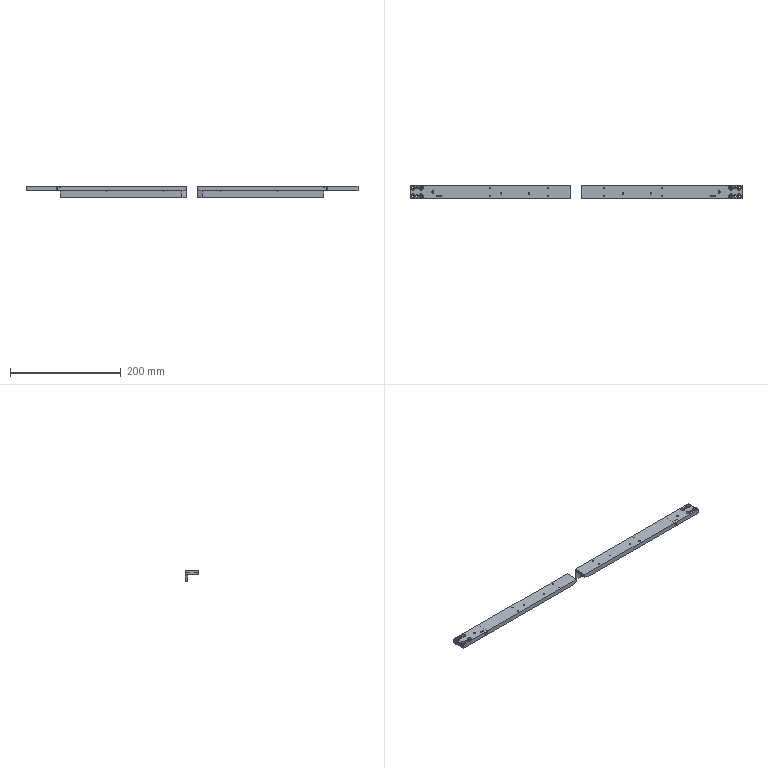Part | 2 solids | 92 faces | box 600 x 25 x 20 mm | volume 138406 mm3 | cylinder 44 | plane 36 | cone 12 | commonest cylinder face diameters 2.5 x16 4.5 x8 8 x8 4 x6 2 x2 3 x2